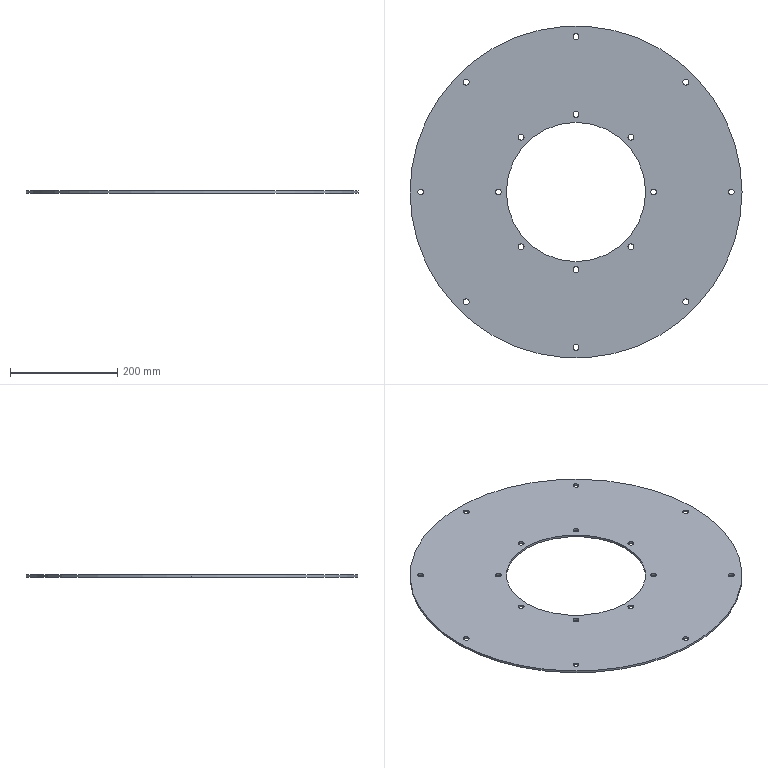Part | STEP file | End disc | 1 solid | 38 faces | box 620 x 620 x 4 mm | volume 989174 mm3 | cylinder 36 | plane 2 | commonest cylinder face diameters 11 x32 260 x2 620 x2